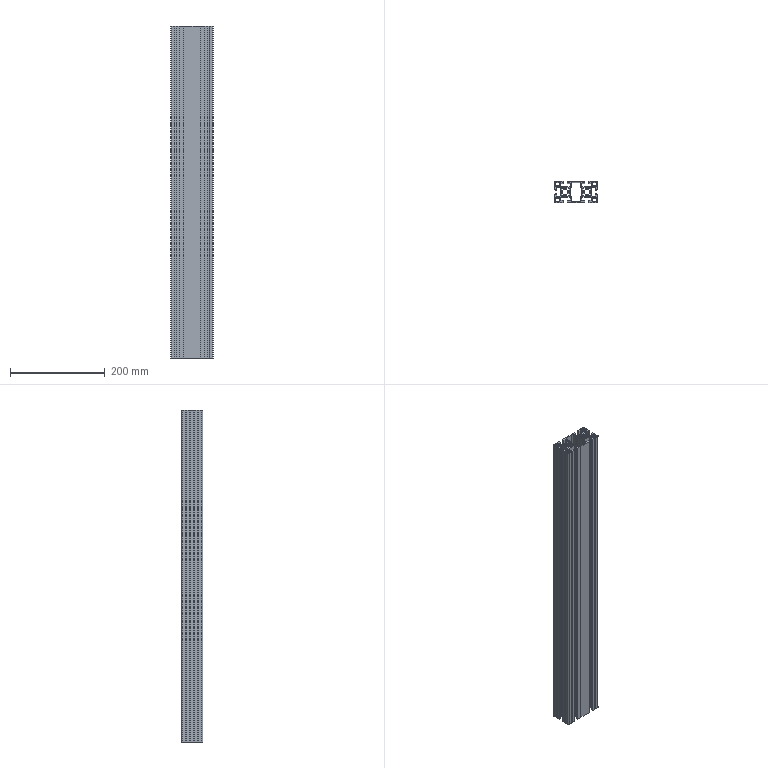Part | STEP file | 4590 aluminium profile (middle longitudinal 3) | 1 solid | 366 faces | box 90 x 45 x 700 mm | volume 820893 mm3 | plane 254 | cylinder 112 | commonest cylinder face diameters 2 x64 8 x20 12 x16 4 x12